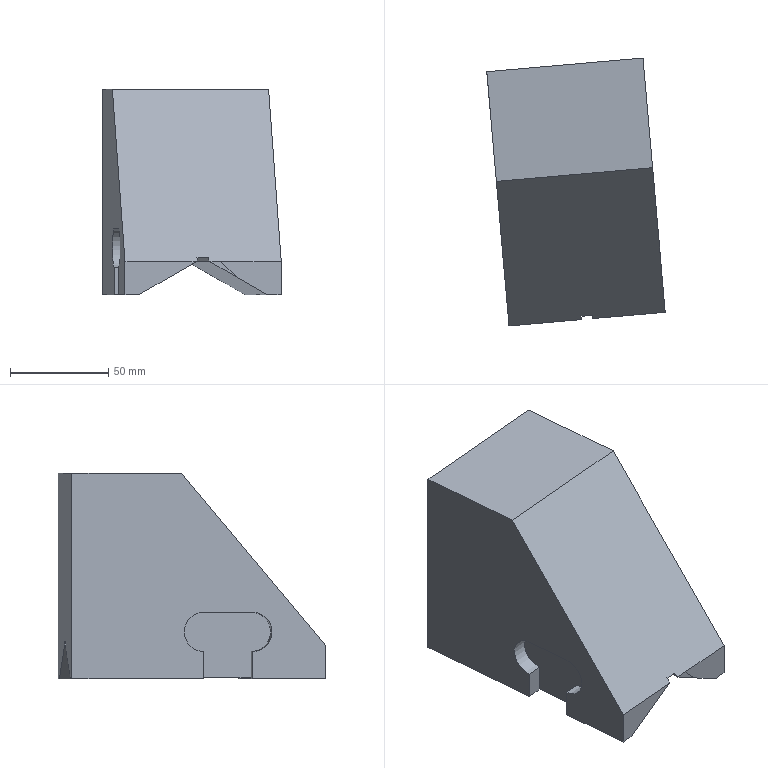Part | NX | features solid 2 | 1 solid | 29 faces | box 91.026 x 136.478 x 105 mm | volume 731515 mm3 | plane 25 | cylinder 4 | commonest cylinder face diameters 20 x4
STEP:
#1=CARTESIAN_POINT('',(746.914,-281.5,-87.));
#2=VERTEX_POINT('',#1);
#3=CARTESIAN_POINT('',(717.581,-284.066,-104.));
#4=VERTEX_POINT('',#3);
#5=CARTESIAN_POINT('',(747.376,-281.46,-86.732));
#6=DIRECTION('',(-0.8627,-0.07548,-0.5));
#7=VECTOR('',#6,1000.);
#8=LINE('',#5,#7);
#9=EDGE_CURVE('',#2,#4,#8,.T.);
#10=ORIENTED_EDGE('',*,*,#9,.F.);
#11=CARTESIAN_POINT('',(741.368,-281.985,-87.));
#12=VERTEX_POINT('',#11);
#13=CARTESIAN_POINT('',(710.517,-284.684,-87.));
#14=DIRECTION('',(-0.9962,-0.08716,0.));
#15=VECTOR('',#14,1000.);
#16=LINE('',#13,#15);
#17=EDGE_CURVE('',#2,#12,#16,.T.);
#18=ORIENTED_EDGE('',*,*,#17,.T.);
#19=CARTESIAN_POINT('',(710.517,-284.684,-87.));
#20=VERTEX_POINT('',#19);
#21=CARTESIAN_POINT('',(790.212,-277.712,-87.));
#22=DIRECTION('',(0.9962,0.08716,0.));
#23=VECTOR('',#22,1000.);
#24=LINE('',#21,#23);
#25=EDGE_CURVE('',#12,#20,#24,.F.);
#26=ORIENTED_EDGE('',*,*,#25,.T.);
#27=CARTESIAN_POINT('',(710.517,-284.684,-104.));
#28=VERTEX_POINT('',#27);
#29=CARTESIAN_POINT('',(710.517,-284.684,-51.5));
#30=DIRECTION('',(0.,0.,-1.));
#31=VECTOR('',#30,1000.);
#32=LINE('',#29,#31);
#33=EDGE_CURVE('',#20,#28,#32,.T.);
#34=ORIENTED_EDGE('',*,*,#33,.T.);
#35=CARTESIAN_POINT('',(710.517,-284.684,-104.));
#36=DIRECTION('',(0.9962,0.08716,0.));
#37=VECTOR('',#36,1000.);
#38=LINE('',#35,#37);
#39=EDGE_CURVE('',#28,#4,#38,.T.);
#40=ORIENTED_EDGE('',*,*,#39,.T.);
#41=EDGE_LOOP('',(#10,#18,#26,#34,#40));
#42=FACE_BOUND('',#41,.T.);
#43=CARTESIAN_POINT('',(710.517,-284.684,-51.5));
#44=DIRECTION('',(0.08716,-0.9962,0.));
#45=DIRECTION('',(0.9962,0.08716,0.));
#46=AXIS2_PLACEMENT_3D('',#43,#44,#45);
#47=PLANE('',#46);
#48=ADVANCED_FACE('',(#42),#47,.T.);
#49=CARTESIAN_POINT('',(759.361,-280.411,-87.));
#50=VERTEX_POINT('',#49);
#51=CARTESIAN_POINT('',(790.212,-277.712,-87.));
#52=VERTEX_POINT('',#51);
#53=CARTESIAN_POINT('',(790.212,-277.712,-87.));
#54=DIRECTION('',(0.9962,0.08716,0.));
#55=VECTOR('',#54,1000.);
#56=LINE('',#53,#55);
#57=EDGE_CURVE('',#50,#52,#56,.T.);
#58=ORIENTED_EDGE('',*,*,#57,.F.);
#59=CARTESIAN_POINT('',(767.237,-279.722,-94.779));
#60=VERTEX_POINT('',#59);
#61=CARTESIAN_POINT('',(716.861,-284.129,-45.027));
#62=DIRECTION('',(0.7101,0.06213,-0.7013));
#63=VECTOR('',#62,1000.);
#64=LINE('',#61,#63);
#65=EDGE_CURVE('',#50,#60,#64,.T.);
#66=ORIENTED_EDGE('',*,*,#65,.T.);
#67=CARTESIAN_POINT('',(783.148,-278.33,-104.));
#68=VERTEX_POINT('',#67);
#69=CARTESIAN_POINT('',(783.148,-278.33,-104.));
#70=DIRECTION('',(-0.8627,-0.07548,0.5));
#71=VECTOR('',#70,1000.);
#72=LINE('',#69,#71);
#73=EDGE_CURVE('',#68,#60,#72,.T.);
#74=ORIENTED_EDGE('',*,*,#73,.F.);
#75=CARTESIAN_POINT('',(790.212,-277.712,-104.));
#76=VERTEX_POINT('',#75);
#77=CARTESIAN_POINT('',(710.517,-284.684,-104.));
#78=DIRECTION('',(0.9962,0.08716,0.));
#79=VECTOR('',#78,1000.);
#80=LINE('',#77,#79);
#81=EDGE_CURVE('',#68,#76,#80,.T.);
#82=ORIENTED_EDGE('',*,*,#81,.T.);
#83=CARTESIAN_POINT('',(790.212,-277.712,-51.5));
#84=DIRECTION('',(0.,0.,1.));
#85=VECTOR('',#84,1000.);
#86=LINE('',#83,#85);
#87=EDGE_CURVE('',#76,#52,#86,.T.);
#88=ORIENTED_EDGE('',*,*,#87,.T.);
#89=EDGE_LOOP('',(#58,#66,#74,#82,#88));
#90=FACE_BOUND('',#89,.T.);
#91=CARTESIAN_POINT('',(710.517,-284.684,-51.5));
#92=DIRECTION('',(0.08716,-0.9962,0.));
#93=DIRECTION('',(0.9962,0.08716,0.));
#94=AXIS2_PLACEMENT_3D('',#91,#92,#93);
#95=PLANE('',#94);
#96=ADVANCED_FACE('',(#90),#95,.T.);
#97=CARTESIAN_POINT('',(747.121,-278.549,-83.518));
#98=VERTEX_POINT('',#97);
#99=CARTESIAN_POINT('',(771.198,-264.169,-68.947));
#100=DIRECTION('',(0.7618,0.455,0.4611));
#101=VECTOR('',#100,1000.);
#102=LINE('',#99,#101);
#103=EDGE_CURVE('',#98,#12,#102,.F.);
#104=ORIENTED_EDGE('',*,*,#103,.F.);
#105=ORIENTED_EDGE('',*,*,#103,.T.);
#106=ORIENTED_EDGE('',*,*,#17,.F.);
#107=CARTESIAN_POINT('',(747.357,-281.236,-86.732));
#108=VERTEX_POINT('',#107);
#109=CARTESIAN_POINT('',(747.29,-281.275,-86.772));
#110=DIRECTION('',(-0.7618,-0.455,-0.4611));
#111=VECTOR('',#110,1000.);
#112=LINE('',#109,#111);
#113=EDGE_CURVE('',#108,#2,#112,.T.);
#114=ORIENTED_EDGE('',*,*,#113,.F.);
#115=CARTESIAN_POINT('',(747.23,-279.788,-85.));
#116=VERTEX_POINT('',#115);
#117=CARTESIAN_POINT('',(747.29,-280.479,-85.826));
#118=DIRECTION('',(0.05602,-0.6403,-0.766));
#119=VECTOR('',#118,1000.);
#120=LINE('',#117,#119);
#121=EDGE_CURVE('',#116,#108,#120,.T.);
#122=ORIENTED_EDGE('',*,*,#121,.F.);
#123=CARTESIAN_POINT('',(753.207,-279.265,-85.));
#124=VERTEX_POINT('',#123);
#125=CARTESIAN_POINT('',(753.207,-279.265,-85.));
#126=DIRECTION('',(-0.9962,-0.08716,0.));
#127=VECTOR('',#126,1000.);
#128=LINE('',#125,#127);
#129=EDGE_CURVE('',#124,#116,#128,.T.);
#130=ORIENTED_EDGE('',*,*,#129,.F.);
#131=CARTESIAN_POINT('',(753.334,-280.713,-86.732));
#132=VERTEX_POINT('',#131);
#133=CARTESIAN_POINT('',(753.353,-280.937,-87.));
#134=DIRECTION('',(0.05602,-0.6403,-0.766));
#135=VECTOR('',#134,1000.);
#136=LINE('',#133,#135);
#137=EDGE_CURVE('',#132,#124,#136,.F.);
#138=ORIENTED_EDGE('',*,*,#137,.F.);
#139=CARTESIAN_POINT('',(753.816,-280.896,-87.));
#140=VERTEX_POINT('',#139);
#141=CARTESIAN_POINT('',(778.011,-290.111,-100.453));
#142=DIRECTION('',(0.8293,-0.3158,-0.4611));
#143=VECTOR('',#142,1000.);
#144=LINE('',#141,#143);
#145=EDGE_CURVE('',#140,#132,#144,.F.);
#146=ORIENTED_EDGE('',*,*,#145,.F.);
#147=CARTESIAN_POINT('',(790.212,-277.712,-87.));
#148=DIRECTION('',(0.9962,0.08716,0.));
#149=VECTOR('',#148,1000.);
#150=LINE('',#147,#149);
#151=EDGE_CURVE('',#50,#140,#150,.F.);
#152=ORIENTED_EDGE('',*,*,#151,.F.);
#153=ORIENTED_EDGE('',*,*,#57,.T.);
#154=CARTESIAN_POINT('',(783.777,-204.152,1.));
#155=VERTEX_POINT('',#154);
#156=CARTESIAN_POINT('',(790.212,-277.712,-87.));
#157=DIRECTION('',(-0.05602,0.6403,0.766));
#158=VECTOR('',#157,1000.);
#159=LINE('',#156,#158);
#160=EDGE_CURVE('',#52,#155,#159,.T.);
#161=ORIENTED_EDGE('',*,*,#160,.T.);
#162=CARTESIAN_POINT('',(704.081,-211.125,1.));
#163=VERTEX_POINT('',#162);
#164=CARTESIAN_POINT('',(704.081,-211.125,1.));
#165=DIRECTION('',(0.9962,0.08716,0.));
#166=VECTOR('',#165,1000.);
#167=LINE('',#164,#166);
#168=EDGE_CURVE('',#163,#155,#167,.T.);
#169=ORIENTED_EDGE('',*,*,#168,.F.);
#170=CARTESIAN_POINT('',(710.517,-284.684,-87.));
#171=DIRECTION('',(0.05602,-0.6403,-0.766));
#172=VECTOR('',#171,1000.);
#173=LINE('',#170,#172);
#174=EDGE_CURVE('',#20,#163,#173,.F.);
#175=ORIENTED_EDGE('',*,*,#174,.F.);
#176=ORIENTED_EDGE('',*,*,#25,.F.);
#177=EDGE_LOOP('',(#104,#105,#106,#114,#122,#130,#138,#146,#152,#153,#161,#169,#175,#176));
#178=FACE_BOUND('',#177,.T.);
#179=CARTESIAN_POINT('',(752.972,-276.578,-81.786));
#180=VERTEX_POINT('',#179);
#181=CARTESIAN_POINT('',(746.995,-277.101,-81.786));
#182=VERTEX_POINT('',#181);
#183=CARTESIAN_POINT('',(789.831,-273.354,-81.786));
#184=DIRECTION('',(0.9962,0.08716,0.));
#185=VECTOR('',#184,1000.);
#186=LINE('',#183,#185);
#187=EDGE_CURVE('',#180,#182,#186,.F.);
#188=ORIENTED_EDGE('',*,*,#187,.T.);
#189=ORIENTED_EDGE('',*,*,#187,.F.);
#190=EDGE_LOOP('',(#188,#189));
#191=FACE_BOUND('',#190,.T.);
#192=CARTESIAN_POINT('',(790.212,-277.712,-87.));
#193=DIRECTION('',(0.06677,-0.7631,0.6428));
#194=DIRECTION('',(-0.05602,0.6403,0.766));
#195=AXIS2_PLACEMENT_3D('',#192,#193,#194);
#196=PLANE('',#195);
#197=ADVANCED_FACE('',(#178,#191),#196,.T.);
#198=CARTESIAN_POINT('',(736.046,-151.954,-86.732));
#199=VERTEX_POINT('',#198);
#200=CARTESIAN_POINT('',(747.376,-281.46,-86.732));
#201=DIRECTION('',(-0.08716,0.9962,0.));
#202=VECTOR('',#201,1000.);
#203=LINE('',#200,#202);
#204=EDGE_CURVE('',#108,#199,#203,.T.);
#205=ORIENTED_EDGE('',*,*,#204,.F.);
#206=ORIENTED_EDGE('',*,*,#113,.T.);
#207=ORIENTED_EDGE('',*,*,#9,.T.);
#208=CARTESIAN_POINT('',(714.313,-246.709,-104.));
#209=VERTEX_POINT('',#208);
#210=CARTESIAN_POINT('',(717.581,-284.066,-104.));
#211=DIRECTION('',(-0.08716,0.9962,0.));
#212=VECTOR('',#211,1000.);
#213=LINE('',#210,#212);
#214=EDGE_CURVE('',#4,#209,#213,.T.);
#215=ORIENTED_EDGE('',*,*,#214,.T.);
#216=CARTESIAN_POINT('',(715.218,-246.63,-103.475));
#217=VERTEX_POINT('',#216);
#218=CARTESIAN_POINT('',(744.108,-244.102,-86.732));
#219=DIRECTION('',(-0.8627,-0.07548,-0.5));
#220=VECTOR('',#219,1000.);
#221=LINE('',#218,#220);
#222=EDGE_CURVE('',#217,#209,#221,.T.);
#223=ORIENTED_EDGE('',*,*,#222,.F.);
#224=CARTESIAN_POINT('',(713.039,-221.725,-103.475));
#225=VERTEX_POINT('',#224);
#226=CARTESIAN_POINT('',(718.486,-283.987,-103.475));
#227=DIRECTION('',(-0.08716,0.9962,0.));
#228=VECTOR('',#227,1000.);
#229=LINE('',#226,#228);
#230=EDGE_CURVE('',#217,#225,#229,.T.);
#231=ORIENTED_EDGE('',*,*,#230,.T.);
#232=CARTESIAN_POINT('',(712.134,-221.804,-104.));
#233=VERTEX_POINT('',#232);
#234=CARTESIAN_POINT('',(741.929,-219.197,-86.732));
#235=DIRECTION('',(-0.8627,-0.07548,-0.5));
#236=VECTOR('',#235,1000.);
#237=LINE('',#234,#236);
#238=EDGE_CURVE('',#225,#233,#237,.T.);
#239=ORIENTED_EDGE('',*,*,#238,.T.);
#240=CARTESIAN_POINT('',(706.251,-154.561,-104.));
#241=VERTEX_POINT('',#240);
#242=CARTESIAN_POINT('',(717.581,-284.066,-104.));
#243=DIRECTION('',(-0.08716,0.9962,0.));
#244=VECTOR('',#243,1000.);
#245=LINE('',#242,#244);
#246=EDGE_CURVE('',#233,#241,#245,.T.);
#247=ORIENTED_EDGE('',*,*,#246,.T.);
#248=CARTESIAN_POINT('',(736.046,-151.954,-86.732));
#249=DIRECTION('',(-0.8627,-0.07548,-0.5));
#250=VECTOR('',#249,1000.);
#251=LINE('',#248,#250);
#252=EDGE_CURVE('',#199,#241,#251,.T.);
#253=ORIENTED_EDGE('',*,*,#252,.F.);
#254=EDGE_LOOP('',(#205,#206,#207,#215,#223,#231,#239,#247,#253));
#255=FACE_BOUND('',#254,.T.);
#256=CARTESIAN_POINT('',(747.376,-281.46,-86.732));
#257=DIRECTION('',(0.4981,0.04358,-0.866));
#258=DIRECTION('',(-0.8627,-0.07548,-0.5));
#259=AXIS2_PLACEMENT_3D('',#256,#257,#258);
#260=PLANE('',#259);
#261=ADVANCED_FACE('',(#255),#260,.T.);
#262=CARTESIAN_POINT('',(742.023,-151.431,-86.732));
#263=VERTEX_POINT('',#262);
#264=CARTESIAN_POINT('',(753.353,-280.937,-86.732));
#265=DIRECTION('',(-0.08716,0.9962,0.));
#266=VECTOR('',#265,1000.);
#267=LINE('',#264,#266);
#268=EDGE_CURVE('',#132,#263,#267,.T.);
#269=ORIENTED_EDGE('',*,*,#268,.F.);
#270=ORIENTED_EDGE('',*,*,#137,.T.);
#271=CARTESIAN_POINT('',(742.023,-151.431,-85.));
#272=VERTEX_POINT('',#271);
#273=CARTESIAN_POINT('',(753.353,-280.937,-85.));
#274=DIRECTION('',(-0.08716,0.9962,0.));
#275=VECTOR('',#274,1000.);
#276=LINE('',#273,#275);
#277=EDGE_CURVE('',#124,#272,#276,.T.);
#278=ORIENTED_EDGE('',*,*,#277,.T.);
#279=CARTESIAN_POINT('',(742.023,-151.431,-86.732));
#280=DIRECTION('',(0.,0.,1.));
#281=VECTOR('',#280,1000.);
#282=LINE('',#279,#281);
#283=EDGE_CURVE('',#263,#272,#282,.T.);
#284=ORIENTED_EDGE('',*,*,#283,.F.);
#285=EDGE_LOOP('',(#269,#270,#278,#284));
#286=FACE_BOUND('',#285,.T.);
#287=CARTESIAN_POINT('',(753.353,-280.937,-86.732));
#288=DIRECTION('',(-0.9962,-0.08716,0.));
#289=DIRECTION('',(0.,0.,1.));
#290=AXIS2_PLACEMENT_3D('',#287,#288,#289);
#291=PLANE('',#290);
#292=ADVANCED_FACE('',(#286),#291,.T.);
#293=ORIENTED_EDGE('',*,*,#277,.F.);
#294=ORIENTED_EDGE('',*,*,#129,.T.);
#295=CARTESIAN_POINT('',(736.046,-151.954,-85.));
#296=VERTEX_POINT('',#295);
#297=CARTESIAN_POINT('',(747.376,-281.46,-85.));
#298=DIRECTION('',(-0.08716,0.9962,0.));
#299=VECTOR('',#298,1000.);
#300=LINE('',#297,#299);
#301=EDGE_CURVE('',#116,#296,#300,.T.);
#302=ORIENTED_EDGE('',*,*,#301,.T.);
#303=CARTESIAN_POINT('',(742.023,-151.431,-85.));
#304=DIRECTION('',(-0.9962,-0.08716,0.));
#305=VECTOR('',#304,1000.);
#306=LINE('',#303,#305);
#307=EDGE_CURVE('',#272,#296,#306,.T.);
#308=ORIENTED_EDGE('',*,*,#307,.F.);
#309=EDGE_LOOP('',(#293,#294,#302,#308));
#310=FACE_BOUND('',#309,.T.);
#311=CARTESIAN_POINT('',(753.353,-280.937,-85.));
#312=DIRECTION('',(0.,0.,-1.));
#313=DIRECTION('',(-0.9962,-0.08716,0.));
#314=AXIS2_PLACEMENT_3D('',#311,#312,#313);
#315=PLANE('',#314);
#316=ADVANCED_FACE('',(#310),#315,.T.);
#317=ORIENTED_EDGE('',*,*,#301,.F.);
#318=ORIENTED_EDGE('',*,*,#121,.T.);
#319=ORIENTED_EDGE('',*,*,#204,.T.);
#320=CARTESIAN_POINT('',(736.046,-151.954,-85.));
#321=DIRECTION('',(0.,0.,-1.));
#322=VECTOR('',#321,1000.);
#323=LINE('',#320,#322);
#324=EDGE_CURVE('',#296,#199,#323,.T.);
#325=ORIENTED_EDGE('',*,*,#324,.F.);
#326=EDGE_LOOP('',(#317,#318,#319,#325));
#327=FACE_BOUND('',#326,.T.);
#328=CARTESIAN_POINT('',(747.376,-281.46,-85.));
#329=DIRECTION('',(0.9962,0.08716,0.));
#330=DIRECTION('',(0.,0.,-1.));
#331=AXIS2_PLACEMENT_3D('',#328,#329,#330);
#332=PLANE('',#331);
#333=ADVANCED_FACE('',(#327),#332,.T.);
#334=CARTESIAN_POINT('',(783.148,-278.33,-104.));
#335=DIRECTION('',(-0.8627,-0.07548,0.5));
#336=VECTOR('',#335,1000.);
#337=LINE('',#334,#336);
#338=EDGE_CURVE('',#60,#140,#337,.T.);
#339=ORIENTED_EDGE('',*,*,#338,.T.);
#340=ORIENTED_EDGE('',*,*,#145,.T.);
#341=ORIENTED_EDGE('',*,*,#268,.T.);
#342=CARTESIAN_POINT('',(771.818,-148.825,-104.));
#343=VERTEX_POINT('',#342);
#344=CARTESIAN_POINT('',(771.818,-148.825,-104.));
#345=DIRECTION('',(-0.8627,-0.07548,0.5));
#346=VECTOR('',#345,1000.);
#347=LINE('',#344,#346);
#348=EDGE_CURVE('',#343,#263,#347,.T.);
#349=ORIENTED_EDGE('',*,*,#348,.F.);
#350=CARTESIAN_POINT('',(777.701,-216.068,-104.));
#351=VERTEX_POINT('',#350);
#352=CARTESIAN_POINT('',(783.148,-278.33,-104.));
#353=DIRECTION('',(-0.08716,0.9962,0.));
#354=VECTOR('',#353,1000.);
#355=LINE('',#352,#354);
#356=EDGE_CURVE('',#351,#343,#355,.T.);
#357=ORIENTED_EDGE('',*,*,#356,.F.);
#358=CARTESIAN_POINT('',(776.796,-216.147,-103.475));
#359=VERTEX_POINT('',#358);
#360=CARTESIAN_POINT('',(777.701,-216.068,-104.));
#361=DIRECTION('',(0.8627,0.07548,-0.5));
#362=VECTOR('',#361,1000.);
#363=LINE('',#360,#362);
#364=EDGE_CURVE('',#359,#351,#363,.T.);
#365=ORIENTED_EDGE('',*,*,#364,.F.);
#366=CARTESIAN_POINT('',(778.975,-241.052,-103.475));
#367=VERTEX_POINT('',#366);
#368=CARTESIAN_POINT('',(782.243,-278.409,-103.475));
#369=DIRECTION('',(0.08716,-0.9962,0.));
#370=VECTOR('',#369,1000.);
#371=LINE('',#368,#370);
#372=EDGE_CURVE('',#359,#367,#371,.T.);
#373=ORIENTED_EDGE('',*,*,#372,.T.);
#374=CARTESIAN_POINT('',(779.88,-240.973,-104.));
#375=VERTEX_POINT('',#374);
#376=CARTESIAN_POINT('',(779.88,-240.973,-104.));
#377=DIRECTION('',(0.8627,0.07548,-0.5));
#378=VECTOR('',#377,1000.);
#379=LINE('',#376,#378);
#380=EDGE_CURVE('',#367,#375,#379,.T.);
#381=ORIENTED_EDGE('',*,*,#380,.T.);
#382=CARTESIAN_POINT('',(783.148,-278.33,-104.));
#383=DIRECTION('',(-0.08716,0.9962,0.));
#384=VECTOR('',#383,1000.);
#385=LINE('',#382,#384);
#386=EDGE_CURVE('',#68,#375,#385,.T.);
#387=ORIENTED_EDGE('',*,*,#386,.F.);
#388=ORIENTED_EDGE('',*,*,#73,.T.);
#389=EDGE_LOOP('',(#339,#340,#341,#349,#357,#365,#373,#381,#387,#388));
#390=FACE_BOUND('',#389,.T.);
#391=CARTESIAN_POINT('',(783.148,-278.33,-104.));
#392=DIRECTION('',(-0.4981,-0.04358,-0.866));
#393=DIRECTION('',(-0.8627,-0.07548,0.5));
#394=AXIS2_PLACEMENT_3D('',#391,#392,#393);
#395=PLANE('',#394);
#396=ADVANCED_FACE('',(#390),#395,.T.);
#397=ORIENTED_EDGE('',*,*,#174,.T.);
#398=CARTESIAN_POINT('',(699.187,-155.179,1.));
#399=VERTEX_POINT('',#398);
#400=CARTESIAN_POINT('',(704.852,-219.932,1.));
#401=DIRECTION('',(0.08716,-0.9962,0.));
#402=VECTOR('',#401,1000.);
#403=LINE('',#400,#402);
#404=EDGE_CURVE('',#399,#163,#403,.T.);
#405=ORIENTED_EDGE('',*,*,#404,.F.);
#406=CARTESIAN_POINT('',(699.187,-155.179,-104.));
#407=VERTEX_POINT('',#406);
#408=CARTESIAN_POINT('',(699.187,-155.179,-51.5));
#409=DIRECTION('',(0.,0.,1.));
#410=VECTOR('',#409,1000.);
#411=LINE('',#408,#410);
#412=EDGE_CURVE('',#407,#399,#411,.T.);
#413=ORIENTED_EDGE('',*,*,#412,.F.);
#414=CARTESIAN_POINT('',(705.07,-222.422,-104.));
#415=VERTEX_POINT('',#414);
#416=CARTESIAN_POINT('',(704.852,-219.932,-104.));
#417=DIRECTION('',(-0.08716,0.9962,0.));
#418=VECTOR('',#417,1000.);
#419=LINE('',#416,#418);
#420=EDGE_CURVE('',#415,#407,#419,.T.);
#421=ORIENTED_EDGE('',*,*,#420,.F.);
#422=CARTESIAN_POINT('',(705.07,-222.422,-90.));
#423=VERTEX_POINT('',#422);
#424=CARTESIAN_POINT('',(705.07,-222.422,-120.));
#425=DIRECTION('',(0.,0.,1.));
#426=VECTOR('',#425,1000.);
#427=LINE('',#424,#426);
#428=EDGE_CURVE('',#415,#423,#427,.T.);
#429=ORIENTED_EDGE('',*,*,#428,.T.);
#430=CARTESIAN_POINT('',(705.07,-222.422,-70.));
#431=VERTEX_POINT('',#430);
#432=CARTESIAN_POINT('',(705.07,-222.422,-80.));
#433=DIRECTION('',(0.9962,0.08716,0.));
#434=DIRECTION('',(-0.07899,0.9029,0.4226));
#435=AXIS2_PLACEMENT_3D('',#432,#433,#434);
#436=CIRCLE('',#435,10.);
#437=EDGE_CURVE('',#423,#431,#436,.T.);
#438=ORIENTED_EDGE('',*,*,#437,.T.);
#439=CARTESIAN_POINT('',(707.249,-247.327,-70.));
#440=VERTEX_POINT('',#439);
#441=CARTESIAN_POINT('',(705.07,-222.422,-70.));
#442=DIRECTION('',(0.08716,-0.9962,0.));
#443=VECTOR('',#442,1000.);
#444=LINE('',#441,#443);
#445=EDGE_CURVE('',#431,#440,#444,.T.);
#446=ORIENTED_EDGE('',*,*,#445,.T.);
#447=CARTESIAN_POINT('',(707.249,-247.327,-90.));
#448=VERTEX_POINT('',#447);
#449=CARTESIAN_POINT('',(707.249,-247.327,-80.));
#450=DIRECTION('',(0.9962,0.08716,0.));
#451=DIRECTION('',(-0.07899,0.9029,0.4226));
#452=AXIS2_PLACEMENT_3D('',#449,#450,#451);
#453=CIRCLE('',#452,10.);
#454=EDGE_CURVE('',#440,#448,#453,.T.);
#455=ORIENTED_EDGE('',*,*,#454,.T.);
#456=CARTESIAN_POINT('',(707.249,-247.327,-104.));
#457=VERTEX_POINT('',#456);
#458=CARTESIAN_POINT('',(707.249,-247.327,-90.));
#459=DIRECTION('',(0.,0.,1.));
#460=VECTOR('',#459,1000.);
#461=LINE('',#458,#460);
#462=EDGE_CURVE('',#457,#448,#461,.T.);
#463=ORIENTED_EDGE('',*,*,#462,.F.);
#464=CARTESIAN_POINT('',(704.852,-219.932,-104.));
#465=DIRECTION('',(-0.08716,0.9962,0.));
#466=VECTOR('',#465,1000.);
#467=LINE('',#464,#466);
#468=EDGE_CURVE('',#28,#457,#467,.T.);
#469=ORIENTED_EDGE('',*,*,#468,.F.);
#470=ORIENTED_EDGE('',*,*,#33,.F.);
#471=EDGE_LOOP('',(#397,#405,#413,#421,#429,#438,#446,#455,#463,#469,#470));
#472=FACE_BOUND('',#471,.T.);
#473=CARTESIAN_POINT('',(704.852,-219.932,-51.5));
#474=DIRECTION('',(-0.9962,-0.08716,0.));
#475=DIRECTION('',(0.08716,-0.9962,0.));
#476=AXIS2_PLACEMENT_3D('',#473,#474,#475);
#477=PLANE('',#476);
#478=ADVANCED_FACE('',(#472),#477,.T.);
#479=ORIENTED_EDGE('',*,*,#246,.F.);
#480=CARTESIAN_POINT('',(705.07,-222.422,-104.));
#481=DIRECTION('',(-0.9962,-0.08716,0.));
#482=VECTOR('',#481,1000.);
#483=LINE('',#480,#482);
#484=EDGE_CURVE('',#233,#415,#483,.T.);
#485=ORIENTED_EDGE('',*,*,#484,.T.);
#486=ORIENTED_EDGE('',*,*,#420,.T.);
#487=CARTESIAN_POINT('',(699.187,-155.179,-104.));
#488=DIRECTION('',(0.9962,0.08716,0.));
#489=VECTOR('',#488,1000.);
#490=LINE('',#487,#489);
#491=EDGE_CURVE('',#407,#241,#490,.T.);
#492=ORIENTED_EDGE('',*,*,#491,.T.);
#493=EDGE_LOOP('',(#479,#485,#486,#492));
#494=FACE_BOUND('',#493,.T.);
#495=CARTESIAN_POINT('',(704.852,-219.932,-104.));
#496=DIRECTION('',(0.,0.,-1.));
#497=DIRECTION('',(-0.9962,-0.08716,0.));
#498=AXIS2_PLACEMENT_3D('',#495,#496,#497);
#499=PLANE('',#498);
#500=ADVANCED_FACE('',(#494),#499,.T.);
#501=ORIENTED_EDGE('',*,*,#386,.T.);
#502=CARTESIAN_POINT('',(786.944,-240.355,-104.));
#503=VERTEX_POINT('',#502);
#504=CARTESIAN_POINT('',(707.249,-247.327,-104.));
#505=DIRECTION('',(0.9962,0.08716,0.));
#506=VECTOR('',#505,1000.);
#507=LINE('',#504,#506);
#508=EDGE_CURVE('',#375,#503,#507,.T.);
#509=ORIENTED_EDGE('',*,*,#508,.T.);
#510=CARTESIAN_POINT('',(784.547,-212.959,-104.));
#511=DIRECTION('',(0.08716,-0.9962,0.));
#512=VECTOR('',#511,1000.);
#513=LINE('',#510,#512);
#514=EDGE_CURVE('',#503,#76,#513,.T.);
#515=ORIENTED_EDGE('',*,*,#514,.T.);
#516=ORIENTED_EDGE('',*,*,#81,.F.);
#517=EDGE_LOOP('',(#501,#509,#515,#516));
#518=FACE_BOUND('',#517,.T.);
#519=CARTESIAN_POINT('',(704.852,-219.932,-104.));
#520=DIRECTION('',(0.,0.,-1.));
#521=DIRECTION('',(-0.9962,-0.08716,0.));
#522=AXIS2_PLACEMENT_3D('',#519,#520,#521);
#523=PLANE('',#522);
#524=ADVANCED_FACE('',(#518),#523,.T.);
#525=CARTESIAN_POINT('',(707.249,-247.327,-104.));
#526=DIRECTION('',(-0.9962,-0.08716,0.));
#527=VECTOR('',#526,1000.);
#528=LINE('',#525,#527);
#529=EDGE_CURVE('',#209,#457,#528,.T.);
#530=ORIENTED_EDGE('',*,*,#529,.F.);
#531=ORIENTED_EDGE('',*,*,#214,.F.);
#532=ORIENTED_EDGE('',*,*,#39,.F.);
#533=ORIENTED_EDGE('',*,*,#468,.T.);
#534=EDGE_LOOP('',(#530,#531,#532,#533));
#535=FACE_BOUND('',#534,.T.);
#536=CARTESIAN_POINT('',(704.852,-219.932,-104.));
#537=DIRECTION('',(0.,0.,-1.));
#538=DIRECTION('',(-0.9962,-0.08716,0.));
#539=AXIS2_PLACEMENT_3D('',#536,#537,#538);
#540=PLANE('',#539);
#541=ADVANCED_FACE('',(#535),#540,.T.);
#542=CARTESIAN_POINT('',(784.765,-215.45,-104.));
#543=VERTEX_POINT('',#542);
#544=CARTESIAN_POINT('',(705.07,-222.422,-104.));
#545=DIRECTION('',(0.9962,0.08716,0.));
#546=VECTOR('',#545,1000.);
#547=LINE('',#544,#546);
#548=EDGE_CURVE('',#351,#543,#547,.T.);
#549=ORIENTED_EDGE('',*,*,#548,.F.);
#550=ORIENTED_EDGE('',*,*,#356,.T.);
#551=CARTESIAN_POINT('',(778.882,-148.207,-104.));
#552=VERTEX_POINT('',#551);
#553=CARTESIAN_POINT('',(699.187,-155.179,-104.));
#554=DIRECTION('',(0.9962,0.08716,0.));
#555=VECTOR('',#554,1000.);
#556=LINE('',#553,#555);
#557=EDGE_CURVE('',#343,#552,#556,.T.);
#558=ORIENTED_EDGE('',*,*,#557,.T.);
#559=CARTESIAN_POINT('',(784.547,-212.959,-104.));
#560=DIRECTION('',(0.08716,-0.9962,0.));
#561=VECTOR('',#560,1000.);
#562=LINE('',#559,#561);
#563=EDGE_CURVE('',#552,#543,#562,.T.);
#564=ORIENTED_EDGE('',*,*,#563,.T.);
#565=EDGE_LOOP('',(#549,#550,#558,#564));
#566=FACE_BOUND('',#565,.T.);
#567=CARTESIAN_POINT('',(704.852,-219.932,-104.));
#568=DIRECTION('',(0.,0.,-1.));
#569=DIRECTION('',(-0.9962,-0.08716,0.));
#570=AXIS2_PLACEMENT_3D('',#567,#568,#569);
#571=PLANE('',#570);
#572=ADVANCED_FACE('',(#566),#571,.T.);
#573=ORIENTED_EDGE('',*,*,#324,.T.);
#574=ORIENTED_EDGE('',*,*,#252,.T.);
#575=ORIENTED_EDGE('',*,*,#491,.F.);
#576=ORIENTED_EDGE('',*,*,#412,.T.);
#577=CARTESIAN_POINT('',(778.882,-148.207,1.));
#578=VERTEX_POINT('',#577);
#579=CARTESIAN_POINT('',(699.187,-155.179,1.));
#580=DIRECTION('',(0.9962,0.08716,0.));
#581=VECTOR('',#580,1000.);
#582=LINE('',#579,#581);
#583=EDGE_CURVE('',#399,#578,#582,.T.);
#584=ORIENTED_EDGE('',*,*,#583,.T.);
#585=CARTESIAN_POINT('',(778.882,-148.207,-51.5));
#586=DIRECTION('',(0.,0.,-1.));
#587=VECTOR('',#586,1000.);
#588=LINE('',#585,#587);
#589=EDGE_CURVE('',#578,#552,#588,.T.);
#590=ORIENTED_EDGE('',*,*,#589,.T.);
#591=ORIENTED_EDGE('',*,*,#557,.F.);
#592=ORIENTED_EDGE('',*,*,#348,.T.);
#593=ORIENTED_EDGE('',*,*,#283,.T.);
#594=ORIENTED_EDGE('',*,*,#307,.T.);
#595=EDGE_LOOP('',(#573,#574,#575,#576,#584,#590,#591,#592,#593,#594));
#596=FACE_BOUND('',#595,.T.);
#597=CARTESIAN_POINT('',(699.187,-155.179,-51.5));
#598=DIRECTION('',(-0.08716,0.9962,0.));
#599=DIRECTION('',(-0.9962,-0.08716,0.));
#600=AXIS2_PLACEMENT_3D('',#597,#598,#599);
#601=PLANE('',#600);
#602=ADVANCED_FACE('',(#596),#601,.T.);
#603=ORIENTED_EDGE('',*,*,#589,.F.);
#604=CARTESIAN_POINT('',(784.547,-212.959,1.));
#605=DIRECTION('',(-0.08716,0.9962,0.));
#606=VECTOR('',#605,1000.);
#607=LINE('',#604,#606);
#608=EDGE_CURVE('',#155,#578,#607,.T.);
#609=ORIENTED_EDGE('',*,*,#608,.F.);
#610=ORIENTED_EDGE('',*,*,#160,.F.);
#611=ORIENTED_EDGE('',*,*,#87,.F.);
#612=ORIENTED_EDGE('',*,*,#514,.F.);
#613=CARTESIAN_POINT('',(786.944,-240.355,-90.));
#614=VERTEX_POINT('',#613);
#615=CARTESIAN_POINT('',(786.944,-240.355,-120.));
#616=DIRECTION('',(0.,0.,1.));
#617=VECTOR('',#616,1000.);
#618=LINE('',#615,#617);
#619=EDGE_CURVE('',#503,#614,#618,.T.);
#620=ORIENTED_EDGE('',*,*,#619,.T.);
#621=CARTESIAN_POINT('',(786.944,-240.355,-70.));
#622=VERTEX_POINT('',#621);
#623=CARTESIAN_POINT('',(786.944,-240.355,-80.));
#624=DIRECTION('',(0.9962,0.08716,0.));
#625=DIRECTION('',(-0.07899,0.9029,0.4226));
#626=AXIS2_PLACEMENT_3D('',#623,#624,#625);
#627=CIRCLE('',#626,10.);
#628=EDGE_CURVE('',#622,#614,#627,.T.);
#629=ORIENTED_EDGE('',*,*,#628,.F.);
#630=CARTESIAN_POINT('',(784.765,-215.45,-70.));
#631=VERTEX_POINT('',#630);
#632=CARTESIAN_POINT('',(786.944,-240.355,-70.));
#633=DIRECTION('',(-0.08716,0.9962,0.));
#634=VECTOR('',#633,1000.);
#635=LINE('',#632,#634);
#636=EDGE_CURVE('',#622,#631,#635,.T.);
#637=ORIENTED_EDGE('',*,*,#636,.T.);
#638=CARTESIAN_POINT('',(784.765,-215.45,-90.));
#639=VERTEX_POINT('',#638);
#640=CARTESIAN_POINT('',(784.765,-215.45,-80.));
#641=DIRECTION('',(0.9962,0.08716,0.));
#642=DIRECTION('',(-0.07899,0.9029,0.4226));
#643=AXIS2_PLACEMENT_3D('',#640,#641,#642);
#644=CIRCLE('',#643,10.);
#645=EDGE_CURVE('',#639,#631,#644,.T.);
#646=ORIENTED_EDGE('',*,*,#645,.F.);
#647=CARTESIAN_POINT('',(784.765,-215.45,-120.));
#648=DIRECTION('',(0.,0.,1.));
#649=VECTOR('',#648,1000.);
#650=LINE('',#647,#649);
#651=EDGE_CURVE('',#543,#639,#650,.T.);
#652=ORIENTED_EDGE('',*,*,#651,.F.);
#653=ORIENTED_EDGE('',*,*,#563,.F.);
#654=EDGE_LOOP('',(#603,#609,#610,#611,#612,#620,#629,#637,#646,#652,#653));
#655=FACE_BOUND('',#654,.T.);
#656=CARTESIAN_POINT('',(784.547,-212.959,-51.5));
#657=DIRECTION('',(0.9962,0.08716,0.));
#658=DIRECTION('',(-0.08716,0.9962,0.));
#659=AXIS2_PLACEMENT_3D('',#656,#657,#658);
#660=PLANE('',#659);
#661=ADVANCED_FACE('',(#655),#660,.T.);
#662=ORIENTED_EDGE('',*,*,#608,.T.);
#663=ORIENTED_EDGE('',*,*,#583,.F.);
#664=ORIENTED_EDGE('',*,*,#404,.T.);
#665=ORIENTED_EDGE('',*,*,#168,.T.);
#666=EDGE_LOOP('',(#662,#663,#664,#665));
#667=FACE_BOUND('',#666,.T.);
#668=CARTESIAN_POINT('',(704.852,-219.932,1.));
#669=DIRECTION('',(0.,0.,1.));
#670=DIRECTION('',(0.9962,0.08716,0.));
#671=AXIS2_PLACEMENT_3D('',#668,#669,#670);
#672=PLANE('',#671);
#673=ADVANCED_FACE('',(#667),#672,.T.);
#674=ORIENTED_EDGE('',*,*,#645,.T.);
#675=CARTESIAN_POINT('',(776.796,-216.147,-70.));
#676=VERTEX_POINT('',#675);
#677=CARTESIAN_POINT('',(776.796,-216.147,-70.));
#678=DIRECTION('',(0.9962,0.08716,0.));
#679=VECTOR('',#678,1000.);
#680=LINE('',#677,#679);
#681=EDGE_CURVE('',#676,#631,#680,.T.);
#682=ORIENTED_EDGE('',*,*,#681,.F.);
#683=CARTESIAN_POINT('',(776.796,-216.147,-90.));
#684=VERTEX_POINT('',#683);
#685=CARTESIAN_POINT('',(776.796,-216.147,-80.));
#686=DIRECTION('',(0.9962,0.08716,0.));
#687=DIRECTION('',(-0.07899,0.9029,0.4226));
#688=AXIS2_PLACEMENT_3D('',#685,#686,#687);
#689=CIRCLE('',#688,10.);
#690=EDGE_CURVE('',#684,#676,#689,.T.);
#691=ORIENTED_EDGE('',*,*,#690,.F.);
#692=CARTESIAN_POINT('',(776.796,-216.147,-90.));
#693=DIRECTION('',(0.9962,0.08716,0.));
#694=VECTOR('',#693,1000.);
#695=LINE('',#692,#694);
#696=EDGE_CURVE('',#684,#639,#695,.T.);
#697=ORIENTED_EDGE('',*,*,#696,.T.);
#698=EDGE_LOOP('',(#674,#682,#691,#697));
#699=FACE_BOUND('',#698,.T.);
#700=CARTESIAN_POINT('',(776.796,-216.147,-80.));
#701=DIRECTION('',(0.9962,0.08716,0.));
#702=DIRECTION('',(-0.07548,0.8627,0.5));
#703=AXIS2_PLACEMENT_3D('',#700,#701,#702);
#704=CYLINDRICAL_SURFACE('',#703,10.);
#705=ADVANCED_FACE('',(#699),#704,.F.);
#706=ORIENTED_EDGE('',*,*,#636,.F.);
#707=CARTESIAN_POINT('',(778.975,-241.052,-70.));
#708=VERTEX_POINT('',#707);
#709=CARTESIAN_POINT('',(778.975,-241.052,-70.));
#710=DIRECTION('',(0.9962,0.08716,0.));
#711=VECTOR('',#710,1000.);
#712=LINE('',#709,#711);
#713=EDGE_CURVE('',#708,#622,#712,.T.);
#714=ORIENTED_EDGE('',*,*,#713,.F.);
#715=CARTESIAN_POINT('',(778.975,-241.052,-70.));
#716=DIRECTION('',(-0.08716,0.9962,0.));
#717=VECTOR('',#716,1000.);
#718=LINE('',#715,#717);
#719=EDGE_CURVE('',#708,#676,#718,.T.);
#720=ORIENTED_EDGE('',*,*,#719,.T.);
#721=ORIENTED_EDGE('',*,*,#681,.T.);
#722=EDGE_LOOP('',(#706,#714,#720,#721));
#723=FACE_BOUND('',#722,.T.);
#724=CARTESIAN_POINT('',(778.975,-241.052,-70.));
#725=DIRECTION('',(0.,0.,-1.));
#726=DIRECTION('',(-0.08716,0.9962,0.));
#727=AXIS2_PLACEMENT_3D('',#724,#725,#726);
#728=PLANE('',#727);
#729=ADVANCED_FACE('',(#723),#728,.T.);
#730=ORIENTED_EDGE('',*,*,#628,.T.);
#731=CARTESIAN_POINT('',(778.975,-241.052,-90.));
#732=VERTEX_POINT('',#731);
#733=CARTESIAN_POINT('',(778.975,-241.052,-90.));
#734=DIRECTION('',(0.9962,0.08716,0.));
#735=VECTOR('',#734,1000.);
#736=LINE('',#733,#735);
#737=EDGE_CURVE('',#732,#614,#736,.T.);
#738=ORIENTED_EDGE('',*,*,#737,.F.);
#739=CARTESIAN_POINT('',(778.975,-241.052,-80.));
#740=DIRECTION('',(0.9962,0.08716,0.));
#741=DIRECTION('',(-0.07899,0.9029,0.4226));
#742=AXIS2_PLACEMENT_3D('',#739,#740,#741);
#743=CIRCLE('',#742,10.);
#744=EDGE_CURVE('',#708,#732,#743,.T.);
#745=ORIENTED_EDGE('',*,*,#744,.F.);
#746=ORIENTED_EDGE('',*,*,#713,.T.);
#747=EDGE_LOOP('',(#730,#738,#745,#746));
#748=FACE_BOUND('',#747,.T.);
#749=CARTESIAN_POINT('',(778.975,-241.052,-80.));
#750=DIRECTION('',(0.9962,0.08716,0.));
#751=DIRECTION('',(-0.07548,0.8627,0.5));
#752=AXIS2_PLACEMENT_3D('',#749,#750,#751);
#753=CYLINDRICAL_SURFACE('',#752,10.);
#754=ADVANCED_FACE('',(#748),#753,.F.);
#755=ORIENTED_EDGE('',*,*,#744,.T.);
#756=CARTESIAN_POINT('',(778.975,-241.052,-120.));
#757=DIRECTION('',(0.,0.,1.));
#758=VECTOR('',#757,1000.);
#759=LINE('',#756,#758);
#760=EDGE_CURVE('',#367,#732,#759,.T.);
#761=ORIENTED_EDGE('',*,*,#760,.F.);
#762=ORIENTED_EDGE('',*,*,#372,.F.);
#763=CARTESIAN_POINT('',(776.796,-216.147,-120.));
#764=DIRECTION('',(0.,0.,1.));
#765=VECTOR('',#764,1000.);
#766=LINE('',#763,#765);
#767=EDGE_CURVE('',#359,#684,#766,.T.);
#768=ORIENTED_EDGE('',*,*,#767,.T.);
#769=ORIENTED_EDGE('',*,*,#690,.T.);
#770=ORIENTED_EDGE('',*,*,#719,.F.);
#771=EDGE_LOOP('',(#755,#761,#762,#768,#769,#770));
#772=FACE_BOUND('',#771,.T.);
#773=CARTESIAN_POINT('',(776.796,-216.147,-80.));
#774=DIRECTION('',(0.9962,0.08716,0.));
#775=DIRECTION('',(-0.07548,0.8627,0.5));
#776=AXIS2_PLACEMENT_3D('',#773,#774,#775);
#777=PLANE('',#776);
#778=ADVANCED_FACE('',(#772),#777,.T.);
#779=ORIENTED_EDGE('',*,*,#548,.T.);
#780=ORIENTED_EDGE('',*,*,#651,.T.);
#781=ORIENTED_EDGE('',*,*,#696,.F.);
#782=ORIENTED_EDGE('',*,*,#767,.F.);
#783=ORIENTED_EDGE('',*,*,#364,.T.);
#784=EDGE_LOOP('',(#779,#780,#781,#782,#783));
#785=FACE_BOUND('',#784,.T.);
#786=CARTESIAN_POINT('',(776.796,-216.147,-120.));
#787=DIRECTION('',(-0.08716,0.9962,0.));
#788=DIRECTION('',(0.,0.,1.));
#789=AXIS2_PLACEMENT_3D('',#786,#787,#788);
#790=PLANE('',#789);
#791=ADVANCED_FACE('',(#785),#790,.F.);
#792=ORIENTED_EDGE('',*,*,#380,.F.);
#793=ORIENTED_EDGE('',*,*,#760,.T.);
#794=ORIENTED_EDGE('',*,*,#737,.T.);
#795=ORIENTED_EDGE('',*,*,#619,.F.);
#796=ORIENTED_EDGE('',*,*,#508,.F.);
#797=EDGE_LOOP('',(#792,#793,#794,#795,#796));
#798=FACE_BOUND('',#797,.T.);
#799=CARTESIAN_POINT('',(778.975,-241.052,-120.));
#800=DIRECTION('',(-0.08716,0.9962,0.));
#801=DIRECTION('',(0.,0.,1.));
#802=AXIS2_PLACEMENT_3D('',#799,#800,#801);
#803=PLANE('',#802);
#804=ADVANCED_FACE('',(#798),#803,.T.);
#805=ORIENTED_EDGE('',*,*,#445,.F.);
#806=CARTESIAN_POINT('',(713.039,-221.725,-70.));
#807=VERTEX_POINT('',#806);
#808=CARTESIAN_POINT('',(713.039,-221.725,-70.));
#809=DIRECTION('',(-0.9962,-0.08716,0.));
#810=VECTOR('',#809,1000.);
#811=LINE('',#808,#810);
#812=EDGE_CURVE('',#807,#431,#811,.T.);
#813=ORIENTED_EDGE('',*,*,#812,.F.);
#814=CARTESIAN_POINT('',(715.218,-246.63,-70.));
#815=VERTEX_POINT('',#814);
#816=CARTESIAN_POINT('',(713.039,-221.725,-70.));
#817=DIRECTION('',(0.08716,-0.9962,0.));
#818=VECTOR('',#817,1000.);
#819=LINE('',#816,#818);
#820=EDGE_CURVE('',#807,#815,#819,.T.);
#821=ORIENTED_EDGE('',*,*,#820,.T.);
#822=CARTESIAN_POINT('',(707.249,-247.327,-70.));
#823=DIRECTION('',(0.9962,0.08716,0.));
#824=VECTOR('',#823,1000.);
#825=LINE('',#822,#824);
#826=EDGE_CURVE('',#440,#815,#825,.T.);
#827=ORIENTED_EDGE('',*,*,#826,.F.);
#828=EDGE_LOOP('',(#805,#813,#821,#827));
#829=FACE_BOUND('',#828,.T.);
#830=CARTESIAN_POINT('',(713.039,-221.725,-70.));
#831=DIRECTION('',(0.,0.,-1.));
#832=DIRECTION('',(-0.08716,0.9962,0.));
#833=AXIS2_PLACEMENT_3D('',#830,#831,#832);
#834=PLANE('',#833);
#835=ADVANCED_FACE('',(#829),#834,.T.);
#836=CARTESIAN_POINT('',(713.039,-221.725,-90.));
#837=VERTEX_POINT('',#836);
#838=CARTESIAN_POINT('',(705.07,-222.422,-90.));
#839=DIRECTION('',(0.9962,0.08716,0.));
#840=VECTOR('',#839,1000.);
#841=LINE('',#838,#840);
#842=EDGE_CURVE('',#423,#837,#841,.T.);
#843=ORIENTED_EDGE('',*,*,#842,.F.);
#844=ORIENTED_EDGE('',*,*,#428,.F.);
#845=ORIENTED_EDGE('',*,*,#484,.F.);
#846=ORIENTED_EDGE('',*,*,#238,.F.);
#847=CARTESIAN_POINT('',(713.039,-221.725,-120.));
#848=DIRECTION('',(0.,0.,1.));
#849=VECTOR('',#848,1000.);
#850=LINE('',#847,#849);
#851=EDGE_CURVE('',#225,#837,#850,.T.);
#852=ORIENTED_EDGE('',*,*,#851,.T.);
#853=EDGE_LOOP('',(#843,#844,#845,#846,#852));
#854=FACE_BOUND('',#853,.T.);
#855=CARTESIAN_POINT('',(713.039,-221.725,-120.));
#856=DIRECTION('',(0.08716,-0.9962,0.));
#857=DIRECTION('',(0.,0.,-1.));
#858=AXIS2_PLACEMENT_3D('',#855,#856,#857);
#859=PLANE('',#858);
#860=ADVANCED_FACE('',(#854),#859,.T.);
#861=ORIENTED_EDGE('',*,*,#462,.T.);
#862=CARTESIAN_POINT('',(715.218,-246.63,-90.));
#863=VERTEX_POINT('',#862);
#864=CARTESIAN_POINT('',(707.249,-247.327,-90.));
#865=DIRECTION('',(0.9962,0.08716,0.));
#866=VECTOR('',#865,1000.);
#867=LINE('',#864,#866);
#868=EDGE_CURVE('',#448,#863,#867,.T.);
#869=ORIENTED_EDGE('',*,*,#868,.T.);
#870=CARTESIAN_POINT('',(715.218,-246.63,-90.));
#871=DIRECTION('',(0.,0.,1.));
#872=VECTOR('',#871,1000.);
#873=LINE('',#870,#872);
#874=EDGE_CURVE('',#217,#863,#873,.T.);
#875=ORIENTED_EDGE('',*,*,#874,.F.);
#876=ORIENTED_EDGE('',*,*,#222,.T.);
#877=ORIENTED_EDGE('',*,*,#529,.T.);
#878=EDGE_LOOP('',(#861,#869,#875,#876,#877));
#879=FACE_BOUND('',#878,.T.);
#880=CARTESIAN_POINT('',(715.218,-246.63,-90.));
#881=DIRECTION('',(0.08716,-0.9962,0.));
#882=DIRECTION('',(0.,0.,-1.));
#883=AXIS2_PLACEMENT_3D('',#880,#881,#882);
#884=PLANE('',#883);
#885=ADVANCED_FACE('',(#879),#884,.F.);
#886=CARTESIAN_POINT('',(715.218,-246.63,-80.));
#887=DIRECTION('',(0.9962,0.08716,0.));
#888=DIRECTION('',(-0.07899,0.9029,0.4226));
#889=AXIS2_PLACEMENT_3D('',#886,#887,#888);
#890=CIRCLE('',#889,10.);
#891=EDGE_CURVE('',#815,#863,#890,.T.);
#892=ORIENTED_EDGE('',*,*,#891,.F.);
#893=ORIENTED_EDGE('',*,*,#820,.F.);
#894=CARTESIAN_POINT('',(713.039,-221.725,-80.));
#895=DIRECTION('',(0.9962,0.08716,0.));
#896=DIRECTION('',(-0.07899,0.9029,0.4226));
#897=AXIS2_PLACEMENT_3D('',#894,#895,#896);
#898=CIRCLE('',#897,10.);
#899=EDGE_CURVE('',#837,#807,#898,.T.);
#900=ORIENTED_EDGE('',*,*,#899,.F.);
#901=ORIENTED_EDGE('',*,*,#851,.F.);
#902=ORIENTED_EDGE('',*,*,#230,.F.);
#903=ORIENTED_EDGE('',*,*,#874,.T.);
#904=EDGE_LOOP('',(#892,#893,#900,#901,#902,#903));
#905=FACE_BOUND('',#904,.T.);
#906=CARTESIAN_POINT('',(713.039,-221.725,-50.));
#907=DIRECTION('',(-0.9962,-0.08716,0.));
#908=DIRECTION('',(-0.07548,0.8627,0.5));
#909=AXIS2_PLACEMENT_3D('',#906,#907,#908);
#910=PLANE('',#909);
#911=ADVANCED_FACE('',(#905),#910,.T.);
#912=ORIENTED_EDGE('',*,*,#891,.T.);
#913=ORIENTED_EDGE('',*,*,#868,.F.);
#914=ORIENTED_EDGE('',*,*,#454,.F.);
#915=ORIENTED_EDGE('',*,*,#826,.T.);
#916=EDGE_LOOP('',(#912,#913,#914,#915));
#917=FACE_BOUND('',#916,.T.);
#918=CARTESIAN_POINT('',(707.249,-247.327,-80.));
#919=DIRECTION('',(0.9962,0.08716,0.));
#920=DIRECTION('',(-0.07548,0.8627,0.5));
#921=AXIS2_PLACEMENT_3D('',#918,#919,#920);
#922=CYLINDRICAL_SURFACE('',#921,10.);
#923=ADVANCED_FACE('',(#917),#922,.F.);
#924=ORIENTED_EDGE('',*,*,#899,.T.);
#925=ORIENTED_EDGE('',*,*,#812,.T.);
#926=ORIENTED_EDGE('',*,*,#437,.F.);
#927=ORIENTED_EDGE('',*,*,#842,.T.);
#928=EDGE_LOOP('',(#924,#925,#926,#927));
#929=FACE_BOUND('',#928,.T.);
#930=CARTESIAN_POINT('',(705.07,-222.422,-80.));
#931=DIRECTION('',(0.9962,0.08716,0.));
#932=DIRECTION('',(-0.07548,0.8627,0.5));
#933=AXIS2_PLACEMENT_3D('',#930,#931,#932);
#934=CYLINDRICAL_SURFACE('',#933,10.);
#935=ADVANCED_FACE('',(#929),#934,.F.);
#936=ORIENTED_EDGE('',*,*,#151,.T.);
#937=ORIENTED_EDGE('',*,*,#338,.F.);
#938=ORIENTED_EDGE('',*,*,#65,.F.);
#939=EDGE_LOOP('',(#936,#937,#938));
#940=FACE_BOUND('',#939,.T.);
#941=CARTESIAN_POINT('',(710.517,-284.684,-51.5));
#942=DIRECTION('',(0.08716,-0.9962,0.));
#943=DIRECTION('',(0.9962,0.08716,0.));
#944=AXIS2_PLACEMENT_3D('',#941,#942,#943);
#945=PLANE('',#944);
#946=ADVANCED_FACE('',(#940),#945,.T.);
#947=CLOSED_SHELL('',(#48,#96,#197,#261,#292,#316,#333,#396,#478,#500,#524,#541,#572,#602,#661,#673,#705,#729,#754,#778,#791,#804,#835,#860,#885,#911,#923,#935,#946));
#948=MANIFOLD_SOLID_BREP('',#947);
#949=(LENGTH_UNIT()NAMED_UNIT(*)SI_UNIT(.MILLI.,.METRE.));
#950=UNCERTAINTY_MEASURE_WITH_UNIT(LENGTH_MEASURE(0.00001),#949,'','');
#951=(NAMED_UNIT(*)PLANE_ANGLE_UNIT()SI_UNIT($,.RADIAN.));
#952=(NAMED_UNIT(*)SI_UNIT($,.STERADIAN.)SOLID_ANGLE_UNIT());
#953=(GEOMETRIC_REPRESENTATION_CONTEXT(3)GLOBAL_UNCERTAINTY_ASSIGNED_CONTEXT((#950))GLOBAL_UNIT_ASSIGNED_CONTEXT((#949,#951,#952))REPRESENTATION_CONTEXT('',''));
#954=ADVANCED_BREP_SHAPE_REPRESENTATION('',(#948),#953);